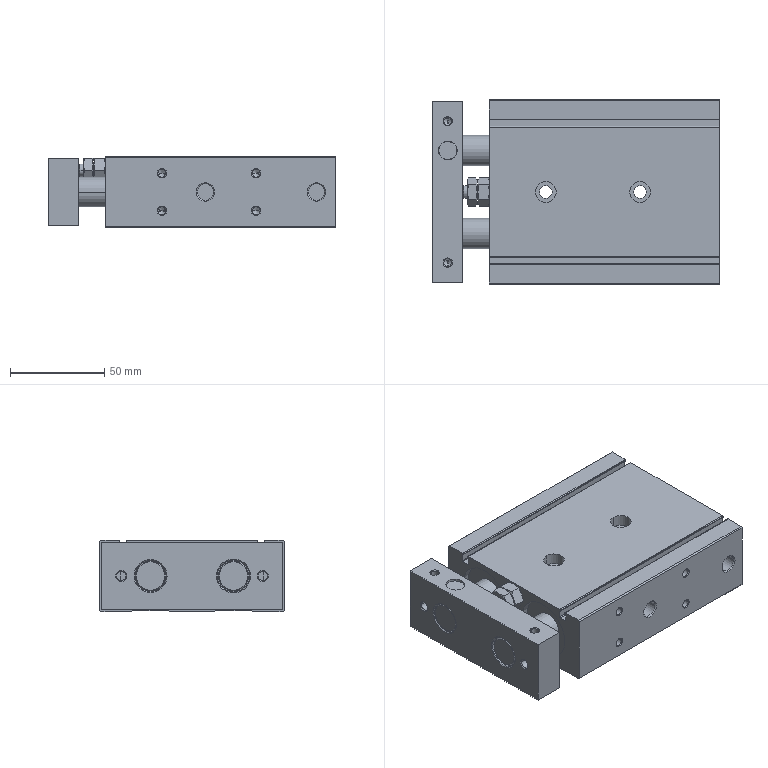Part | SolidWorks | 2 solids | 275 faces | box 152 x 98 x 38 mm | volume 442498 mm3 | cone 100 | cylinder 98 | plane 77 | commonest cylinder face diameters 4.134 x20 0.8 x12 16 x12 32 x12 8.566 x8 0.4 x4